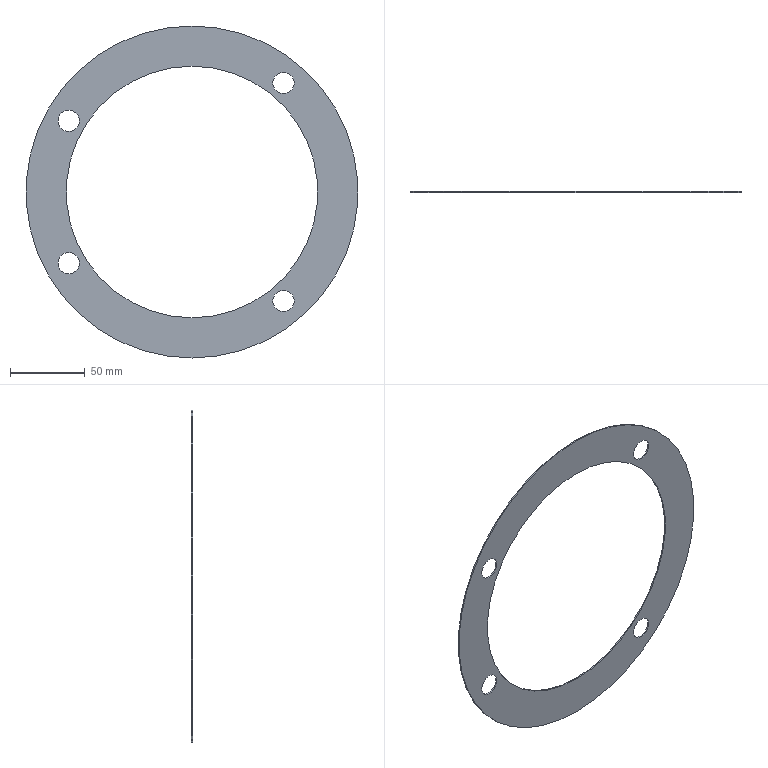Part | SolidWorks | features HoleWzd 2, 3DProfileFeature 1, Extrusion 1, MirrorPattern 1 | 1 solid | 14 faces | box 222.25 x 0.7938 x 222.25 mm | volume 12605 mm3 | cylinder 12 | plane 2 | commonest cylinder face diameters 14.287 x4 14.288 x4 168.4 x2 222.25 x2
STEP:
#1=CARTESIAN_POINT('',(-82.499,0.7937,54.769));
#2=VERTEX_POINT('',#1);
#3=CARTESIAN_POINT('',(-82.499,0.7937,40.481));
#4=VERTEX_POINT('',#3);
#5=CARTESIAN_POINT('',(-82.499,0.7937,47.625));
#6=DIRECTION('',(0.,-1.,0.));
#7=DIRECTION('',(0.,0.,-1.));
#8=AXIS2_PLACEMENT_3D('',#5,#6,#7);
#9=CIRCLE('',#8,7.144);
#10=EDGE_CURVE('',#2,#4,#9,.T.);
#11=ORIENTED_EDGE('',*,*,#10,.F.);
#12=CARTESIAN_POINT('',(-82.499,0.,54.769));
#13=VERTEX_POINT('',#12);
#14=CARTESIAN_POINT('',(-82.499,0.,54.769));
#15=DIRECTION('',(0.,-1.,0.));
#16=VECTOR('',#15,1000.);
#17=LINE('',#14,#16);
#18=EDGE_CURVE('',#2,#13,#17,.T.);
#19=ORIENTED_EDGE('',*,*,#18,.T.);
#20=CARTESIAN_POINT('',(-82.499,0.,40.481));
#21=VERTEX_POINT('',#20);
#22=CARTESIAN_POINT('',(-82.499,0.,47.625));
#23=DIRECTION('',(0.,-1.,0.));
#24=DIRECTION('',(0.,0.,-1.));
#25=AXIS2_PLACEMENT_3D('',#22,#23,#24);
#26=CIRCLE('',#25,7.144);
#27=EDGE_CURVE('',#13,#21,#26,.T.);
#28=ORIENTED_EDGE('',*,*,#27,.T.);
#29=CARTESIAN_POINT('',(-82.499,0.,40.481));
#30=DIRECTION('',(0.,-1.,0.));
#31=VECTOR('',#30,1000.);
#32=LINE('',#29,#31);
#33=EDGE_CURVE('',#4,#21,#32,.T.);
#34=ORIENTED_EDGE('',*,*,#33,.F.);
#35=EDGE_LOOP('',(#11,#19,#28,#34));
#36=FACE_OUTER_BOUND('',#35,.T.);
#37=CARTESIAN_POINT('',(-82.499,0.,47.625));
#38=DIRECTION('',(0.,-1.,0.));
#39=DIRECTION('',(0.,0.,-1.));
#40=AXIS2_PLACEMENT_3D('',#37,#38,#39);
#41=CYLINDRICAL_SURFACE('',#40,7.144);
#42=ADVANCED_FACE('',(#36),#41,.F.);
#43=CARTESIAN_POINT('',(61.215,0.,65.83));
#44=VERTEX_POINT('',#43);
#45=CARTESIAN_POINT('',(61.215,0.,80.118));
#46=VERTEX_POINT('',#45);
#47=CARTESIAN_POINT('',(61.215,0.,72.974));
#48=DIRECTION('',(0.,1.,0.));
#49=DIRECTION('',(0.,0.,1.));
#50=AXIS2_PLACEMENT_3D('',#47,#48,#49);
#51=CIRCLE('',#50,7.144);
#52=EDGE_CURVE('',#44,#46,#51,.T.);
#53=ORIENTED_EDGE('',*,*,#52,.F.);
#54=CARTESIAN_POINT('',(61.215,0.7938,65.83));
#55=VERTEX_POINT('',#54);
#56=CARTESIAN_POINT('',(61.215,0.7937,65.83));
#57=DIRECTION('',(0.,1.,0.));
#58=VECTOR('',#57,1000.);
#59=LINE('',#56,#58);
#60=EDGE_CURVE('',#44,#55,#59,.T.);
#61=ORIENTED_EDGE('',*,*,#60,.T.);
#62=CARTESIAN_POINT('',(61.215,0.7938,80.118));
#63=VERTEX_POINT('',#62);
#64=CARTESIAN_POINT('',(61.215,0.7938,72.974));
#65=DIRECTION('',(0.,1.,0.));
#66=DIRECTION('',(0.,0.,1.));
#67=AXIS2_PLACEMENT_3D('',#64,#65,#66);
#68=CIRCLE('',#67,7.144);
#69=EDGE_CURVE('',#55,#63,#68,.T.);
#70=ORIENTED_EDGE('',*,*,#69,.T.);
#71=CARTESIAN_POINT('',(61.215,0.7937,80.118));
#72=DIRECTION('',(0.,1.,0.));
#73=VECTOR('',#72,1000.);
#74=LINE('',#71,#73);
#75=EDGE_CURVE('',#46,#63,#74,.T.);
#76=ORIENTED_EDGE('',*,*,#75,.F.);
#77=EDGE_LOOP('',(#53,#61,#70,#76));
#78=FACE_OUTER_BOUND('',#77,.T.);
#79=CARTESIAN_POINT('',(61.215,0.7937,72.974));
#80=DIRECTION('',(0.,1.,0.));
#81=DIRECTION('',(0.,0.,1.));
#82=AXIS2_PLACEMENT_3D('',#79,#80,#81);
#83=CYLINDRICAL_SURFACE('',#82,7.144);
#84=ADVANCED_FACE('',(#78),#83,.F.);
#85=CARTESIAN_POINT('',(-82.499,0.7937,-40.481));
#86=VERTEX_POINT('',#85);
#87=CARTESIAN_POINT('',(-82.499,0.7937,-54.769));
#88=VERTEX_POINT('',#87);
#89=CARTESIAN_POINT('',(-82.499,0.7937,-47.625));
#90=DIRECTION('',(0.,-1.,0.));
#91=DIRECTION('',(0.,0.,-1.));
#92=AXIS2_PLACEMENT_3D('',#89,#90,#91);
#93=CIRCLE('',#92,7.144);
#94=EDGE_CURVE('',#86,#88,#93,.T.);
#95=ORIENTED_EDGE('',*,*,#94,.F.);
#96=CARTESIAN_POINT('',(-82.499,0.,-40.481));
#97=VERTEX_POINT('',#96);
#98=CARTESIAN_POINT('',(-82.499,0.,-40.481));
#99=DIRECTION('',(0.,-1.,0.));
#100=VECTOR('',#99,1000.);
#101=LINE('',#98,#100);
#102=EDGE_CURVE('',#86,#97,#101,.T.);
#103=ORIENTED_EDGE('',*,*,#102,.T.);
#104=CARTESIAN_POINT('',(-82.499,0.,-54.769));
#105=VERTEX_POINT('',#104);
#106=CARTESIAN_POINT('',(-82.499,0.,-47.625));
#107=DIRECTION('',(0.,-1.,0.));
#108=DIRECTION('',(0.,0.,-1.));
#109=AXIS2_PLACEMENT_3D('',#106,#107,#108);
#110=CIRCLE('',#109,7.144);
#111=EDGE_CURVE('',#97,#105,#110,.T.);
#112=ORIENTED_EDGE('',*,*,#111,.T.);
#113=CARTESIAN_POINT('',(-82.499,0.,-54.769));
#114=DIRECTION('',(0.,-1.,0.));
#115=VECTOR('',#114,1000.);
#116=LINE('',#113,#115);
#117=EDGE_CURVE('',#88,#105,#116,.T.);
#118=ORIENTED_EDGE('',*,*,#117,.F.);
#119=EDGE_LOOP('',(#95,#103,#112,#118));
#120=FACE_OUTER_BOUND('',#119,.T.);
#121=CARTESIAN_POINT('',(-82.499,0.,-47.625));
#122=DIRECTION('',(0.,-1.,0.));
#123=DIRECTION('',(0.,0.,-1.));
#124=AXIS2_PLACEMENT_3D('',#121,#122,#123);
#125=CYLINDRICAL_SURFACE('',#124,7.144);
#126=ADVANCED_FACE('',(#120),#125,.F.);
#127=CARTESIAN_POINT('',(61.215,0.,-80.118));
#128=VERTEX_POINT('',#127);
#129=CARTESIAN_POINT('',(61.215,0.,-65.83));
#130=VERTEX_POINT('',#129);
#131=CARTESIAN_POINT('',(61.215,0.,-72.974));
#132=DIRECTION('',(0.,1.,0.));
#133=DIRECTION('',(0.,0.,1.));
#134=AXIS2_PLACEMENT_3D('',#131,#132,#133);
#135=CIRCLE('',#134,7.144);
#136=EDGE_CURVE('',#128,#130,#135,.T.);
#137=ORIENTED_EDGE('',*,*,#136,.F.);
#138=CARTESIAN_POINT('',(61.215,0.7938,-80.118));
#139=VERTEX_POINT('',#138);
#140=CARTESIAN_POINT('',(61.215,0.7937,-80.118));
#141=DIRECTION('',(0.,1.,0.));
#142=VECTOR('',#141,1000.);
#143=LINE('',#140,#142);
#144=EDGE_CURVE('',#128,#139,#143,.T.);
#145=ORIENTED_EDGE('',*,*,#144,.T.);
#146=CARTESIAN_POINT('',(61.215,0.7938,-65.83));
#147=VERTEX_POINT('',#146);
#148=CARTESIAN_POINT('',(61.215,0.7938,-72.974));
#149=DIRECTION('',(0.,1.,0.));
#150=DIRECTION('',(0.,0.,1.));
#151=AXIS2_PLACEMENT_3D('',#148,#149,#150);
#152=CIRCLE('',#151,7.144);
#153=EDGE_CURVE('',#139,#147,#152,.T.);
#154=ORIENTED_EDGE('',*,*,#153,.T.);
#155=CARTESIAN_POINT('',(61.215,0.7937,-65.83));
#156=DIRECTION('',(0.,1.,0.));
#157=VECTOR('',#156,1000.);
#158=LINE('',#155,#157);
#159=EDGE_CURVE('',#130,#147,#158,.T.);
#160=ORIENTED_EDGE('',*,*,#159,.F.);
#161=EDGE_LOOP('',(#137,#145,#154,#160));
#162=FACE_OUTER_BOUND('',#161,.T.);
#163=CARTESIAN_POINT('',(61.215,0.7937,-72.974));
#164=DIRECTION('',(0.,1.,0.));
#165=DIRECTION('',(0.,0.,1.));
#166=AXIS2_PLACEMENT_3D('',#163,#164,#165);
#167=CYLINDRICAL_SURFACE('',#166,7.144);
#168=ADVANCED_FACE('',(#162),#167,.F.);
#169=CARTESIAN_POINT('',(0.,0.7937,-84.2));
#170=VERTEX_POINT('',#169);
#171=CARTESIAN_POINT('',(0.,0.7937,84.2));
#172=VERTEX_POINT('',#171);
#173=CARTESIAN_POINT('',(0.,0.7937,0.));
#174=DIRECTION('',(0.,1.,0.));
#175=DIRECTION('',(0.,0.,1.));
#176=AXIS2_PLACEMENT_3D('',#173,#174,#175);
#177=CIRCLE('',#176,84.2);
#178=EDGE_CURVE('',#170,#172,#177,.T.);
#179=ORIENTED_EDGE('',*,*,#178,.T.);
#180=CARTESIAN_POINT('',(0.,0.,84.2));
#181=VERTEX_POINT('',#180);
#182=CARTESIAN_POINT('',(0.,0.7937,84.2));
#183=DIRECTION('',(0.,-1.,0.));
#184=VECTOR('',#183,1000.);
#185=LINE('',#182,#184);
#186=EDGE_CURVE('',#172,#181,#185,.T.);
#187=ORIENTED_EDGE('',*,*,#186,.T.);
#188=CARTESIAN_POINT('',(0.,0.,-84.2));
#189=VERTEX_POINT('',#188);
#190=CARTESIAN_POINT('',(0.,0.,0.));
#191=DIRECTION('',(0.,1.,0.));
#192=DIRECTION('',(0.,0.,1.));
#193=AXIS2_PLACEMENT_3D('',#190,#191,#192);
#194=CIRCLE('',#193,84.2);
#195=EDGE_CURVE('',#189,#181,#194,.T.);
#196=ORIENTED_EDGE('',*,*,#195,.F.);
#197=CARTESIAN_POINT('',(0.,0.7937,-84.2));
#198=DIRECTION('',(0.,-1.,0.));
#199=VECTOR('',#198,1000.);
#200=LINE('',#197,#199);
#201=EDGE_CURVE('',#170,#189,#200,.T.);
#202=ORIENTED_EDGE('',*,*,#201,.F.);
#203=EDGE_LOOP('',(#179,#187,#196,#202));
#204=FACE_OUTER_BOUND('',#203,.T.);
#205=CARTESIAN_POINT('',(0.,0.7937,0.));
#206=DIRECTION('',(0.,-1.,0.));
#207=DIRECTION('',(0.,0.,-1.));
#208=AXIS2_PLACEMENT_3D('',#205,#206,#207);
#209=CYLINDRICAL_SURFACE('',#208,84.2);
#210=ADVANCED_FACE('',(#204),#209,.F.);
#211=CARTESIAN_POINT('',(0.,0.7937,111.125));
#212=VERTEX_POINT('',#211);
#213=CARTESIAN_POINT('',(0.,0.7937,-111.125));
#214=VERTEX_POINT('',#213);
#215=CARTESIAN_POINT('',(0.,0.7937,0.));
#216=DIRECTION('',(0.,1.,0.));
#217=DIRECTION('',(0.,0.,1.));
#218=AXIS2_PLACEMENT_3D('',#215,#216,#217);
#219=CIRCLE('',#218,111.125);
#220=EDGE_CURVE('',#212,#214,#219,.T.);
#221=ORIENTED_EDGE('',*,*,#220,.F.);
#222=CARTESIAN_POINT('',(0.,0.,111.125));
#223=VERTEX_POINT('',#222);
#224=CARTESIAN_POINT('',(0.,0.7937,111.125));
#225=DIRECTION('',(0.,-1.,0.));
#226=VECTOR('',#225,1000.);
#227=LINE('',#224,#226);
#228=EDGE_CURVE('',#212,#223,#227,.T.);
#229=ORIENTED_EDGE('',*,*,#228,.T.);
#230=CARTESIAN_POINT('',(0.,0.,-111.125));
#231=VERTEX_POINT('',#230);
#232=CARTESIAN_POINT('',(0.,0.,0.));
#233=DIRECTION('',(0.,1.,0.));
#234=DIRECTION('',(0.,0.,1.));
#235=AXIS2_PLACEMENT_3D('',#232,#233,#234);
#236=CIRCLE('',#235,111.125);
#237=EDGE_CURVE('',#223,#231,#236,.T.);
#238=ORIENTED_EDGE('',*,*,#237,.T.);
#239=CARTESIAN_POINT('',(0.,0.7937,-111.125));
#240=DIRECTION('',(0.,-1.,0.));
#241=VECTOR('',#240,1000.);
#242=LINE('',#239,#241);
#243=EDGE_CURVE('',#214,#231,#242,.T.);
#244=ORIENTED_EDGE('',*,*,#243,.F.);
#245=EDGE_LOOP('',(#221,#229,#238,#244));
#246=FACE_OUTER_BOUND('',#245,.T.);
#247=CARTESIAN_POINT('',(0.,0.7937,0.));
#248=DIRECTION('',(0.,-1.,0.));
#249=DIRECTION('',(0.,0.,-1.));
#250=AXIS2_PLACEMENT_3D('',#247,#248,#249);
#251=CYLINDRICAL_SURFACE('',#250,111.125);
#252=ADVANCED_FACE('',(#246),#251,.T.);
#253=ORIENTED_EDGE('',*,*,#195,.T.);
#254=CARTESIAN_POINT('',(0.,0.,0.));
#255=DIRECTION('',(0.,1.,0.));
#256=DIRECTION('',(0.,0.,1.));
#257=AXIS2_PLACEMENT_3D('',#254,#255,#256);
#258=CIRCLE('',#257,84.2);
#259=EDGE_CURVE('',#181,#189,#258,.T.);
#260=ORIENTED_EDGE('',*,*,#259,.T.);
#261=EDGE_LOOP('',(#253,#260));
#262=FACE_BOUND('',#261,.T.);
#263=CARTESIAN_POINT('',(0.,0.,0.));
#264=DIRECTION('',(0.,1.,0.));
#265=DIRECTION('',(0.,0.,1.));
#266=AXIS2_PLACEMENT_3D('',#263,#264,#265);
#267=CIRCLE('',#266,111.125);
#268=EDGE_CURVE('',#231,#223,#267,.T.);
#269=ORIENTED_EDGE('',*,*,#268,.F.);
#270=ORIENTED_EDGE('',*,*,#237,.F.);
#271=EDGE_LOOP('',(#269,#270));
#272=FACE_OUTER_BOUND('',#271,.T.);
#273=CARTESIAN_POINT('',(61.215,0.,-72.974));
#274=DIRECTION('',(0.,1.,0.));
#275=DIRECTION('',(0.,0.,1.));
#276=AXIS2_PLACEMENT_3D('',#273,#274,#275);
#277=CIRCLE('',#276,7.144);
#278=EDGE_CURVE('',#130,#128,#277,.T.);
#279=ORIENTED_EDGE('',*,*,#278,.T.);
#280=ORIENTED_EDGE('',*,*,#136,.T.);
#281=EDGE_LOOP('',(#279,#280));
#282=FACE_BOUND('',#281,.T.);
#283=CARTESIAN_POINT('',(-82.499,0.,-47.625));
#284=DIRECTION('',(0.,-1.,0.));
#285=DIRECTION('',(0.,0.,-1.));
#286=AXIS2_PLACEMENT_3D('',#283,#284,#285);
#287=CIRCLE('',#286,7.144);
#288=EDGE_CURVE('',#105,#97,#287,.T.);
#289=ORIENTED_EDGE('',*,*,#288,.F.);
#290=ORIENTED_EDGE('',*,*,#111,.F.);
#291=EDGE_LOOP('',(#289,#290));
#292=FACE_BOUND('',#291,.T.);
#293=CARTESIAN_POINT('',(61.215,0.,72.974));
#294=DIRECTION('',(0.,1.,0.));
#295=DIRECTION('',(0.,0.,1.));
#296=AXIS2_PLACEMENT_3D('',#293,#294,#295);
#297=CIRCLE('',#296,7.144);
#298=EDGE_CURVE('',#46,#44,#297,.T.);
#299=ORIENTED_EDGE('',*,*,#298,.T.);
#300=ORIENTED_EDGE('',*,*,#52,.T.);
#301=EDGE_LOOP('',(#299,#300));
#302=FACE_BOUND('',#301,.T.);
#303=CARTESIAN_POINT('',(-82.499,0.,47.625));
#304=DIRECTION('',(0.,-1.,0.));
#305=DIRECTION('',(0.,0.,-1.));
#306=AXIS2_PLACEMENT_3D('',#303,#304,#305);
#307=CIRCLE('',#306,7.144);
#308=EDGE_CURVE('',#21,#13,#307,.T.);
#309=ORIENTED_EDGE('',*,*,#308,.F.);
#310=ORIENTED_EDGE('',*,*,#27,.F.);
#311=EDGE_LOOP('',(#309,#310));
#312=FACE_BOUND('',#311,.T.);
#313=CARTESIAN_POINT('',(0.,0.,0.));
#314=DIRECTION('',(0.,1.,0.));
#315=DIRECTION('',(0.,0.,1.));
#316=AXIS2_PLACEMENT_3D('',#313,#314,#315);
#317=PLANE('',#316);
#318=ADVANCED_FACE('',(#262,#272,#282,#292,#302,#312),#317,.F.);
#319=CARTESIAN_POINT('',(-82.499,0.7937,47.625));
#320=DIRECTION('',(0.,-1.,0.));
#321=DIRECTION('',(0.,0.,-1.));
#322=AXIS2_PLACEMENT_3D('',#319,#320,#321);
#323=CIRCLE('',#322,7.144);
#324=EDGE_CURVE('',#4,#2,#323,.T.);
#325=ORIENTED_EDGE('',*,*,#324,.T.);
#326=ORIENTED_EDGE('',*,*,#10,.T.);
#327=EDGE_LOOP('',(#325,#326));
#328=FACE_BOUND('',#327,.T.);
#329=CARTESIAN_POINT('',(61.215,0.7938,72.974));
#330=DIRECTION('',(0.,1.,0.));
#331=DIRECTION('',(0.,0.,1.));
#332=AXIS2_PLACEMENT_3D('',#329,#330,#331);
#333=CIRCLE('',#332,7.144);
#334=EDGE_CURVE('',#63,#55,#333,.T.);
#335=ORIENTED_EDGE('',*,*,#334,.F.);
#336=ORIENTED_EDGE('',*,*,#69,.F.);
#337=EDGE_LOOP('',(#335,#336));
#338=FACE_BOUND('',#337,.T.);
#339=CARTESIAN_POINT('',(-82.499,0.7937,-47.625));
#340=DIRECTION('',(0.,-1.,0.));
#341=DIRECTION('',(0.,0.,-1.));
#342=AXIS2_PLACEMENT_3D('',#339,#340,#341);
#343=CIRCLE('',#342,7.144);
#344=EDGE_CURVE('',#88,#86,#343,.T.);
#345=ORIENTED_EDGE('',*,*,#344,.T.);
#346=ORIENTED_EDGE('',*,*,#94,.T.);
#347=EDGE_LOOP('',(#345,#346));
#348=FACE_BOUND('',#347,.T.);
#349=CARTESIAN_POINT('',(61.215,0.7938,-72.974));
#350=DIRECTION('',(0.,1.,0.));
#351=DIRECTION('',(0.,0.,1.));
#352=AXIS2_PLACEMENT_3D('',#349,#350,#351);
#353=CIRCLE('',#352,7.144);
#354=EDGE_CURVE('',#147,#139,#353,.T.);
#355=ORIENTED_EDGE('',*,*,#354,.F.);
#356=ORIENTED_EDGE('',*,*,#153,.F.);
#357=EDGE_LOOP('',(#355,#356));
#358=FACE_BOUND('',#357,.T.);
#359=CARTESIAN_POINT('',(0.,0.7937,0.));
#360=DIRECTION('',(0.,1.,0.));
#361=DIRECTION('',(0.,0.,1.));
#362=AXIS2_PLACEMENT_3D('',#359,#360,#361);
#363=CIRCLE('',#362,111.125);
#364=EDGE_CURVE('',#214,#212,#363,.T.);
#365=ORIENTED_EDGE('',*,*,#364,.T.);
#366=ORIENTED_EDGE('',*,*,#220,.T.);
#367=EDGE_LOOP('',(#365,#366));
#368=FACE_OUTER_BOUND('',#367,.T.);
#369=ORIENTED_EDGE('',*,*,#178,.F.);
#370=CARTESIAN_POINT('',(0.,0.7937,0.));
#371=DIRECTION('',(0.,1.,0.));
#372=DIRECTION('',(0.,0.,1.));
#373=AXIS2_PLACEMENT_3D('',#370,#371,#372);
#374=CIRCLE('',#373,84.2);
#375=EDGE_CURVE('',#172,#170,#374,.T.);
#376=ORIENTED_EDGE('',*,*,#375,.F.);
#377=EDGE_LOOP('',(#369,#376));
#378=FACE_BOUND('',#377,.T.);
#379=CARTESIAN_POINT('',(0.,0.7937,0.));
#380=DIRECTION('',(0.,1.,0.));
#381=DIRECTION('',(0.,0.,1.));
#382=AXIS2_PLACEMENT_3D('',#379,#380,#381);
#383=PLANE('',#382);
#384=ADVANCED_FACE('',(#328,#338,#348,#358,#368,#378),#383,.T.);
#385=ORIENTED_EDGE('',*,*,#228,.F.);
#386=ORIENTED_EDGE('',*,*,#364,.F.);
#387=ORIENTED_EDGE('',*,*,#243,.T.);
#388=ORIENTED_EDGE('',*,*,#268,.T.);
#389=EDGE_LOOP('',(#385,#386,#387,#388));
#390=FACE_OUTER_BOUND('',#389,.T.);
#391=CARTESIAN_POINT('',(0.,0.7937,0.));
#392=DIRECTION('',(0.,-1.,0.));
#393=DIRECTION('',(0.,0.,-1.));
#394=AXIS2_PLACEMENT_3D('',#391,#392,#393);
#395=CYLINDRICAL_SURFACE('',#394,111.125);
#396=ADVANCED_FACE('',(#390),#395,.T.);
#397=ORIENTED_EDGE('',*,*,#186,.F.);
#398=ORIENTED_EDGE('',*,*,#375,.T.);
#399=ORIENTED_EDGE('',*,*,#201,.T.);
#400=ORIENTED_EDGE('',*,*,#259,.F.);
#401=EDGE_LOOP('',(#397,#398,#399,#400));
#402=FACE_OUTER_BOUND('',#401,.T.);
#403=CARTESIAN_POINT('',(0.,0.7937,0.));
#404=DIRECTION('',(0.,-1.,0.));
#405=DIRECTION('',(0.,0.,-1.));
#406=AXIS2_PLACEMENT_3D('',#403,#404,#405);
#407=CYLINDRICAL_SURFACE('',#406,84.2);
#408=ADVANCED_FACE('',(#402),#407,.F.);
#409=ORIENTED_EDGE('',*,*,#144,.F.);
#410=ORIENTED_EDGE('',*,*,#278,.F.);
#411=ORIENTED_EDGE('',*,*,#159,.T.);
#412=ORIENTED_EDGE('',*,*,#354,.T.);
#413=EDGE_LOOP('',(#409,#410,#411,#412));
#414=FACE_OUTER_BOUND('',#413,.T.);
#415=CARTESIAN_POINT('',(61.215,0.7937,-72.974));
#416=DIRECTION('',(0.,1.,0.));
#417=DIRECTION('',(0.,0.,1.));
#418=AXIS2_PLACEMENT_3D('',#415,#416,#417);
#419=CYLINDRICAL_SURFACE('',#418,7.144);
#420=ADVANCED_FACE('',(#414),#419,.F.);
#421=ORIENTED_EDGE('',*,*,#102,.F.);
#422=ORIENTED_EDGE('',*,*,#344,.F.);
#423=ORIENTED_EDGE('',*,*,#117,.T.);
#424=ORIENTED_EDGE('',*,*,#288,.T.);
#425=EDGE_LOOP('',(#421,#422,#423,#424));
#426=FACE_OUTER_BOUND('',#425,.T.);
#427=CARTESIAN_POINT('',(-82.499,0.,-47.625));
#428=DIRECTION('',(0.,-1.,0.));
#429=DIRECTION('',(0.,0.,-1.));
#430=AXIS2_PLACEMENT_3D('',#427,#428,#429);
#431=CYLINDRICAL_SURFACE('',#430,7.144);
#432=ADVANCED_FACE('',(#426),#431,.F.);
#433=ORIENTED_EDGE('',*,*,#60,.F.);
#434=ORIENTED_EDGE('',*,*,#298,.F.);
#435=ORIENTED_EDGE('',*,*,#75,.T.);
#436=ORIENTED_EDGE('',*,*,#334,.T.);
#437=EDGE_LOOP('',(#433,#434,#435,#436));
#438=FACE_OUTER_BOUND('',#437,.T.);
#439=CARTESIAN_POINT('',(61.215,0.7937,72.974));
#440=DIRECTION('',(0.,1.,0.));
#441=DIRECTION('',(0.,0.,1.));
#442=AXIS2_PLACEMENT_3D('',#439,#440,#441);
#443=CYLINDRICAL_SURFACE('',#442,7.144);
#444=ADVANCED_FACE('',(#438),#443,.F.);
#445=ORIENTED_EDGE('',*,*,#18,.F.);
#446=ORIENTED_EDGE('',*,*,#324,.F.);
#447=ORIENTED_EDGE('',*,*,#33,.T.);
#448=ORIENTED_EDGE('',*,*,#308,.T.);
#449=EDGE_LOOP('',(#445,#446,#447,#448));
#450=FACE_OUTER_BOUND('',#449,.T.);
#451=CARTESIAN_POINT('',(-82.499,0.,47.625));
#452=DIRECTION('',(0.,-1.,0.));
#453=DIRECTION('',(0.,0.,-1.));
#454=AXIS2_PLACEMENT_3D('',#451,#452,#453);
#455=CYLINDRICAL_SURFACE('',#454,7.144);
#456=ADVANCED_FACE('',(#450),#455,.F.);
#457=CLOSED_SHELL('',(#42,#84,#126,#168,#210,#252,#318,#384,#396,#408,#420,#432,#444,#456));
#458=MANIFOLD_SOLID_BREP('',#457);
#459=CARTESIAN_POINT('',(0.,0.,0.));
#460=DIRECTION('',(0.,0.,1.));
#461=DIRECTION('',(1.,0.,0.));
#462=AXIS2_PLACEMENT_3D('',#459,#460,#461);
#463=(LENGTH_UNIT()NAMED_UNIT(*)SI_UNIT(.MILLI.,.METRE.));
#464=UNCERTAINTY_MEASURE_WITH_UNIT(LENGTH_MEASURE(0.00001),#463,'','');
#465=(NAMED_UNIT(*)PLANE_ANGLE_UNIT()SI_UNIT($,.RADIAN.));
#466=(NAMED_UNIT(*)SI_UNIT($,.STERADIAN.)SOLID_ANGLE_UNIT());
#467=(GEOMETRIC_REPRESENTATION_CONTEXT(3)GLOBAL_UNCERTAINTY_ASSIGNED_CONTEXT((#464))GLOBAL_UNIT_ASSIGNED_CONTEXT((#463,#465,#466))REPRESENTATION_CONTEXT('',''));
#468=ADVANCED_BREP_SHAPE_REPRESENTATION('',(#458,#462),#467);